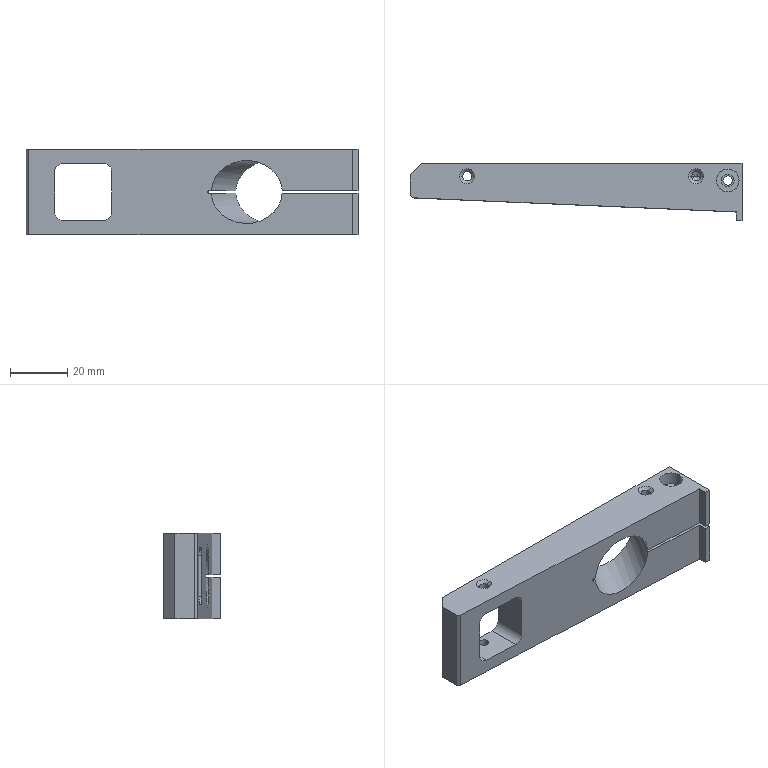Part | SolidWorks | features HoleWzd 6, ICE 4, Chamfer 3, Extrusion 1, Fillet 1, MirrorPattern 1, RevCut 1 | 1 solid | 84 faces | box 116 x 20 x 30 mm | volume 36706 mm3 | cylinder 35 | plane 27 | cone 22 | commonest cylinder face diameters 3.3 x14 6 x8 2.5 x4 4.5 x2 5 x2 8 x2